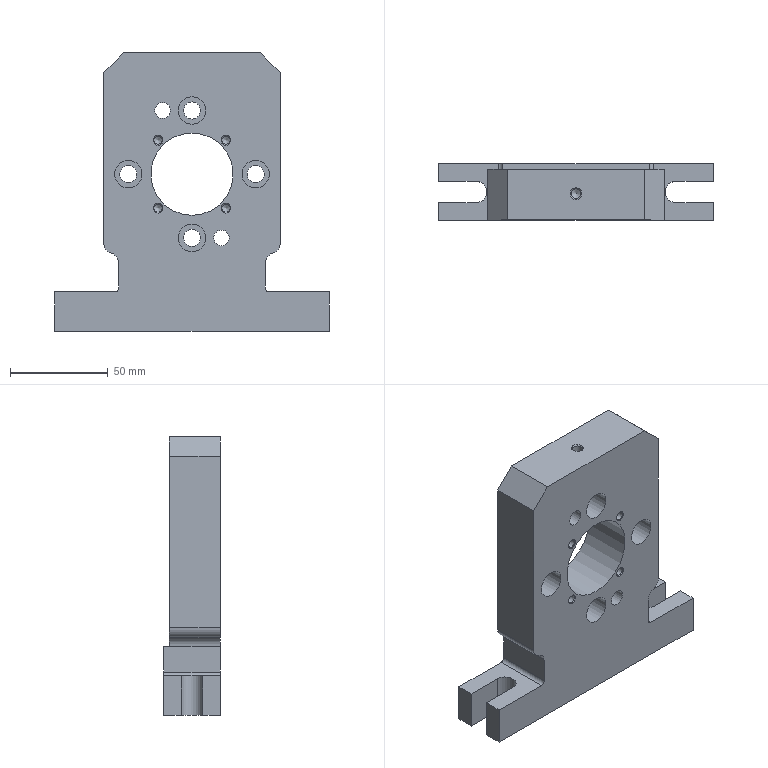Part | STEP file | 冲床-300配套压波_id918_x_t | 1 solid | 60 faces | box 140 x 29 x 142 mm | volume 300034 mm3 | plane 26 | cylinder 24 | cone 10 | commonest cylinder face diameters 4.2 x4 8.7 x4 10 x4 14 x4 4 x2 8 x2